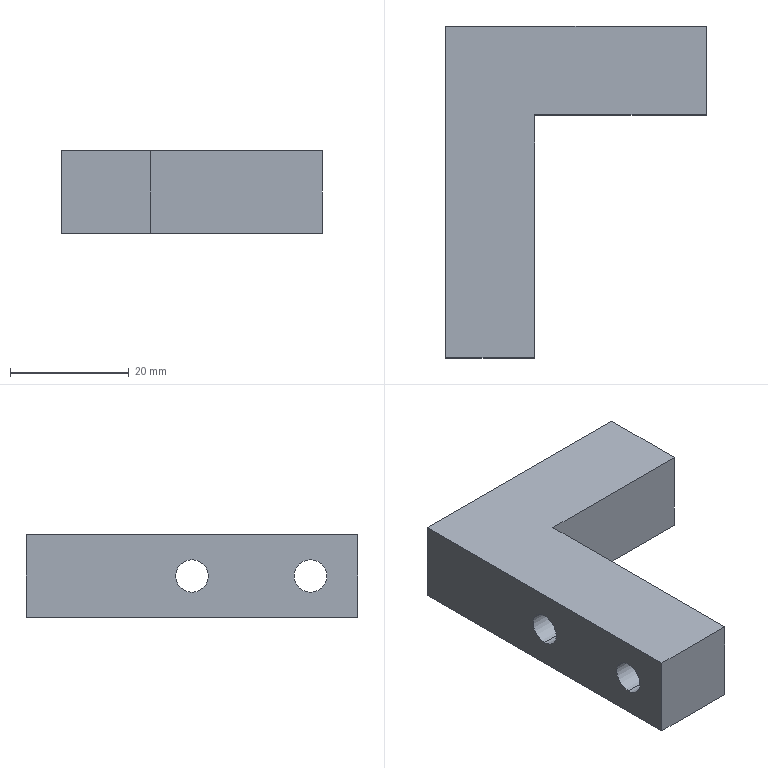Part | STEP file | PN_0017 fixing block | 1 solid | 20 faces | box 44 x 56 x 14 mm | volume 16926 mm3 | cylinder 8 | plane 8 | cone 4 | commonest cylinder face diameters 3.3 x4 5.5 x4
STEP:
#1=CARTESIAN_POINT('',(0.,0.,0.));
#2=DIRECTION('',(0.,0.,1.));
#3=DIRECTION('',(1.,0.,0.));
#4=AXIS2_PLACEMENT_3D('',#1,#2,#3);
#5=CARTESIAN_POINT('',(9.,44.,1.65));
#6=VERTEX_POINT('',#5);
#7=CARTESIAN_POINT('',(9.,56.,1.65));
#8=VERTEX_POINT('',#7);
#9=CARTESIAN_POINT('',(9.,56.,1.65));
#10=DIRECTION('',(0.,1.,0.));
#11=VECTOR('',#10,1.);
#12=LINE('',#9,#11);
#13=CARTESIAN_POINT('',(9.,56.,0.));
#14=DIRECTION('',(0.,1.,0.));
#15=DIRECTION('',(0.,0.,1.));
#16=AXIS2_PLACEMENT_3D('',#13,#14,#15);
#17=CYLINDRICAL_SURFACE('',#16,1.65);
#18=CARTESIAN_POINT('',(6.283,0.));
#19=DIRECTION('',(0.,1.));
#20=VECTOR('',#19,1.);
#21=LINE('',#18,#20);
#22=(GEOMETRIC_REPRESENTATION_CONTEXT(2)PARAMETRIC_REPRESENTATION_CONTEXT()REPRESENTATION_CONTEXT('',''));
#23=DEFINITIONAL_REPRESENTATION('',(#21),#22);
#24=PCURVE('',#17,#23);
#25=CARTESIAN_POINT('',(9.,56.,0.));
#26=DIRECTION('',(0.,1.,0.));
#27=DIRECTION('',(0.,0.,1.));
#28=AXIS2_PLACEMENT_3D('',#25,#26,#27);
#29=CYLINDRICAL_SURFACE('',#28,1.65);
#30=CARTESIAN_POINT('',(0.,0.));
#31=DIRECTION('',(0.,1.));
#32=VECTOR('',#31,1.);
#33=LINE('',#30,#32);
#34=(GEOMETRIC_REPRESENTATION_CONTEXT(2)PARAMETRIC_REPRESENTATION_CONTEXT()REPRESENTATION_CONTEXT('',''));
#35=DEFINITIONAL_REPRESENTATION('',(#33),#34);
#36=PCURVE('',#29,#35);
#37=SURFACE_CURVE('',#12,(#24,#36),.PCURVE_S1.);
#38=EDGE_CURVE('',#6,#8,#37,.T.);
#39=ORIENTED_EDGE('',*,*,#38,.T.);
#40=CARTESIAN_POINT('',(9.,56.,-1.65));
#41=VERTEX_POINT('',#40);
#42=CARTESIAN_POINT('',(9.,56.,0.));
#43=DIRECTION('',(0.,1.,0.));
#44=DIRECTION('',(0.,0.,1.));
#45=AXIS2_PLACEMENT_3D('',#42,#43,#44);
#46=CIRCLE('',#45,1.65);
#47=CARTESIAN_POINT('',(0.,0.));
#48=DIRECTION('',(1.,0.));
#49=VECTOR('',#48,1.);
#50=LINE('',#47,#49);
#51=(GEOMETRIC_REPRESENTATION_CONTEXT(2)PARAMETRIC_REPRESENTATION_CONTEXT()REPRESENTATION_CONTEXT('',''));
#52=DEFINITIONAL_REPRESENTATION('',(#50),#51);
#53=PCURVE('',#17,#52);
#54=CARTESIAN_POINT('',(0.,56.,7.));
#55=DIRECTION('',(0.,-1.,0.));
#56=DIRECTION('',(0.,0.,-1.));
#57=AXIS2_PLACEMENT_3D('',#54,#55,#56);
#58=PLANE('',#57);
#59=CARTESIAN_POINT('',(5.35,9.));
#60=CARTESIAN_POINT('',(5.35,11.858));
#61=CARTESIAN_POINT('',(7.825,10.429));
#62=CARTESIAN_POINT('',(10.3,9.));
#63=CARTESIAN_POINT('',(7.825,7.571));
#64=CARTESIAN_POINT('',(5.35,6.142));
#65=CARTESIAN_POINT('',(5.35,9.));
#66=(BOUNDED_CURVE()B_SPLINE_CURVE(2,(#59,#60,#61,#62,#63,#64,#65),.UNSPECIFIED.,.T.,.F.)B_SPLINE_CURVE_WITH_KNOTS((1,2,2,2,2,1),(-2.094,0.,2.094,4.189,6.283,8.378),.UNSPECIFIED.)CURVE()GEOMETRIC_REPRESENTATION_ITEM()RATIONAL_B_SPLINE_CURVE((1.,0.5,1.,0.5,1.,0.5,1.))REPRESENTATION_ITEM(''));
#67=(GEOMETRIC_REPRESENTATION_CONTEXT(2)PARAMETRIC_REPRESENTATION_CONTEXT()REPRESENTATION_CONTEXT('',''));
#68=DEFINITIONAL_REPRESENTATION('',(#66),#67);
#69=PCURVE('',#58,#68);
#70=SURFACE_CURVE('',#46,(#53,#69),.PCURVE_S1.);
#71=EDGE_CURVE('',#41,#8,#70,.T.);
#72=ORIENTED_EDGE('',*,*,#71,.F.);
#73=CARTESIAN_POINT('',(9.,44.,-1.65));
#74=VERTEX_POINT('',#73);
#75=CARTESIAN_POINT('',(9.,56.,-1.65));
#76=DIRECTION('',(0.,1.,0.));
#77=VECTOR('',#76,1.);
#78=LINE('',#75,#77);
#79=CARTESIAN_POINT('',(3.142,0.));
#80=DIRECTION('',(0.,1.));
#81=VECTOR('',#80,1.);
#82=LINE('',#79,#81);
#83=(GEOMETRIC_REPRESENTATION_CONTEXT(2)PARAMETRIC_REPRESENTATION_CONTEXT()REPRESENTATION_CONTEXT('',''));
#84=DEFINITIONAL_REPRESENTATION('',(#82),#83);
#85=PCURVE('',#17,#84);
#86=CARTESIAN_POINT('',(3.142,0.));
#87=DIRECTION('',(0.,1.));
#88=VECTOR('',#87,1.);
#89=LINE('',#86,#88);
#90=(GEOMETRIC_REPRESENTATION_CONTEXT(2)PARAMETRIC_REPRESENTATION_CONTEXT()REPRESENTATION_CONTEXT('',''));
#91=DEFINITIONAL_REPRESENTATION('',(#89),#90);
#92=PCURVE('',#29,#91);
#93=SURFACE_CURVE('',#78,(#85,#92),.PCURVE_S1.);
#94=EDGE_CURVE('',#74,#41,#93,.T.);
#95=ORIENTED_EDGE('',*,*,#94,.F.);
#96=CARTESIAN_POINT('',(9.,44.,0.));
#97=DIRECTION('',(0.,1.,0.));
#98=DIRECTION('',(0.,0.,1.));
#99=AXIS2_PLACEMENT_3D('',#96,#97,#98);
#100=CIRCLE('',#99,1.65);
#101=CARTESIAN_POINT('',(0.,-12.));
#102=DIRECTION('',(1.,0.));
#103=VECTOR('',#102,1.);
#104=LINE('',#101,#103);
#105=(GEOMETRIC_REPRESENTATION_CONTEXT(2)PARAMETRIC_REPRESENTATION_CONTEXT()REPRESENTATION_CONTEXT('',''));
#106=DEFINITIONAL_REPRESENTATION('',(#104),#105);
#107=PCURVE('',#17,#106);
#108=CARTESIAN_POINT('',(9.,44.,0.));
#109=DIRECTION('',(0.,1.,0.));
#110=DIRECTION('',(0.,0.,1.));
#111=AXIS2_PLACEMENT_3D('',#108,#109,#110);
#112=CONICAL_SURFACE('',#111,1.65,1.03);
#113=CARTESIAN_POINT('',(0.,0.));
#114=DIRECTION('',(1.,0.));
#115=VECTOR('',#114,1.);
#116=LINE('',#113,#115);
#117=(GEOMETRIC_REPRESENTATION_CONTEXT(2)PARAMETRIC_REPRESENTATION_CONTEXT()REPRESENTATION_CONTEXT('',''));
#118=DEFINITIONAL_REPRESENTATION('',(#116),#117);
#119=PCURVE('',#112,#118);
#120=SURFACE_CURVE('',#100,(#107,#119),.PCURVE_S1.);
#121=EDGE_CURVE('',#74,#6,#120,.T.);
#122=ORIENTED_EDGE('',*,*,#121,.T.);
#123=EDGE_LOOP('',(#39,#72,#95,#122));
#124=FACE_BOUND('',#123,.F.);
#125=ADVANCED_FACE('',(#124),#17,.F.);
#126=ORIENTED_EDGE('',*,*,#121,.F.);
#127=CARTESIAN_POINT('',(9.,43.009,0.));
#128=VERTEX_POINT('',#127);
#129=CARTESIAN_POINT('',(9.,44.,-1.65));
#130=DIRECTION('',(0.,0.515,-0.8572));
#131=VECTOR('',#130,1.);
#132=LINE('',#129,#131);
#133=CARTESIAN_POINT('',(3.142,0.));
#134=DIRECTION('',(0.,1.));
#135=VECTOR('',#134,1.);
#136=LINE('',#133,#135);
#137=(GEOMETRIC_REPRESENTATION_CONTEXT(2)PARAMETRIC_REPRESENTATION_CONTEXT()REPRESENTATION_CONTEXT('',''));
#138=DEFINITIONAL_REPRESENTATION('',(#136),#137);
#139=PCURVE('',#112,#138);
#140=CARTESIAN_POINT('',(9.,44.,0.));
#141=DIRECTION('',(0.,1.,0.));
#142=DIRECTION('',(0.,0.,1.));
#143=AXIS2_PLACEMENT_3D('',#140,#141,#142);
#144=CONICAL_SURFACE('',#143,1.65,1.03);
#145=CARTESIAN_POINT('',(3.142,0.));
#146=DIRECTION('',(0.,1.));
#147=VECTOR('',#146,1.);
#148=LINE('',#145,#147);
#149=(GEOMETRIC_REPRESENTATION_CONTEXT(2)PARAMETRIC_REPRESENTATION_CONTEXT()REPRESENTATION_CONTEXT('',''));
#150=DEFINITIONAL_REPRESENTATION('',(#148),#149);
#151=PCURVE('',#144,#150);
#152=SURFACE_CURVE('',#132,(#139,#151),.PCURVE_S1.);
#153=EDGE_CURVE('',#128,#74,#152,.T.);
#154=ORIENTED_EDGE('',*,*,#153,.F.);
#155=CARTESIAN_POINT('',(9.,44.,1.65));
#156=DIRECTION('',(0.,0.515,0.8572));
#157=VECTOR('',#156,1.);
#158=LINE('',#155,#157);
#159=CARTESIAN_POINT('',(6.283,0.));
#160=DIRECTION('',(0.,1.));
#161=VECTOR('',#160,1.);
#162=LINE('',#159,#161);
#163=(GEOMETRIC_REPRESENTATION_CONTEXT(2)PARAMETRIC_REPRESENTATION_CONTEXT()REPRESENTATION_CONTEXT('',''));
#164=DEFINITIONAL_REPRESENTATION('',(#162),#163);
#165=PCURVE('',#112,#164);
#166=CARTESIAN_POINT('',(0.,0.));
#167=DIRECTION('',(0.,1.));
#168=VECTOR('',#167,1.);
#169=LINE('',#166,#168);
#170=(GEOMETRIC_REPRESENTATION_CONTEXT(2)PARAMETRIC_REPRESENTATION_CONTEXT()REPRESENTATION_CONTEXT('',''));
#171=DEFINITIONAL_REPRESENTATION('',(#169),#170);
#172=PCURVE('',#144,#171);
#173=SURFACE_CURVE('',#158,(#165,#172),.PCURVE_S1.);
#174=EDGE_CURVE('',#128,#6,#173,.T.);
#175=ORIENTED_EDGE('',*,*,#174,.T.);
#176=EDGE_LOOP('',(#126,#154,#175));
#177=FACE_BOUND('',#176,.F.);
#178=ADVANCED_FACE('',(#177),#112,.F.);
#179=CARTESIAN_POINT('',(29.,44.,1.65));
#180=VERTEX_POINT('',#179);
#181=CARTESIAN_POINT('',(29.,56.,1.65));
#182=VERTEX_POINT('',#181);
#183=CARTESIAN_POINT('',(29.,56.,1.65));
#184=DIRECTION('',(0.,1.,0.));
#185=VECTOR('',#184,1.);
#186=LINE('',#183,#185);
#187=CARTESIAN_POINT('',(29.,56.,0.));
#188=DIRECTION('',(0.,1.,0.));
#189=DIRECTION('',(0.,0.,1.));
#190=AXIS2_PLACEMENT_3D('',#187,#188,#189);
#191=CYLINDRICAL_SURFACE('',#190,1.65);
#192=CARTESIAN_POINT('',(6.283,0.));
#193=DIRECTION('',(0.,1.));
#194=VECTOR('',#193,1.);
#195=LINE('',#192,#194);
#196=(GEOMETRIC_REPRESENTATION_CONTEXT(2)PARAMETRIC_REPRESENTATION_CONTEXT()REPRESENTATION_CONTEXT('',''));
#197=DEFINITIONAL_REPRESENTATION('',(#195),#196);
#198=PCURVE('',#191,#197);
#199=CARTESIAN_POINT('',(29.,56.,0.));
#200=DIRECTION('',(0.,1.,0.));
#201=DIRECTION('',(0.,0.,1.));
#202=AXIS2_PLACEMENT_3D('',#199,#200,#201);
#203=CYLINDRICAL_SURFACE('',#202,1.65);
#204=CARTESIAN_POINT('',(0.,0.));
#205=DIRECTION('',(0.,1.));
#206=VECTOR('',#205,1.);
#207=LINE('',#204,#206);
#208=(GEOMETRIC_REPRESENTATION_CONTEXT(2)PARAMETRIC_REPRESENTATION_CONTEXT()REPRESENTATION_CONTEXT('',''));
#209=DEFINITIONAL_REPRESENTATION('',(#207),#208);
#210=PCURVE('',#203,#209);
#211=SURFACE_CURVE('',#186,(#198,#210),.PCURVE_S1.);
#212=EDGE_CURVE('',#180,#182,#211,.T.);
#213=ORIENTED_EDGE('',*,*,#212,.T.);
#214=CARTESIAN_POINT('',(29.,56.,-1.65));
#215=VERTEX_POINT('',#214);
#216=CARTESIAN_POINT('',(29.,56.,0.));
#217=DIRECTION('',(0.,1.,0.));
#218=DIRECTION('',(0.,0.,1.));
#219=AXIS2_PLACEMENT_3D('',#216,#217,#218);
#220=CIRCLE('',#219,1.65);
#221=CARTESIAN_POINT('',(0.,0.));
#222=DIRECTION('',(1.,0.));
#223=VECTOR('',#222,1.);
#224=LINE('',#221,#223);
#225=(GEOMETRIC_REPRESENTATION_CONTEXT(2)PARAMETRIC_REPRESENTATION_CONTEXT()REPRESENTATION_CONTEXT('',''));
#226=DEFINITIONAL_REPRESENTATION('',(#224),#225);
#227=PCURVE('',#191,#226);
#228=CARTESIAN_POINT('',(5.35,29.));
#229=CARTESIAN_POINT('',(5.35,31.858));
#230=CARTESIAN_POINT('',(7.825,30.429));
#231=CARTESIAN_POINT('',(10.3,29.));
#232=CARTESIAN_POINT('',(7.825,27.571));
#233=CARTESIAN_POINT('',(5.35,26.142));
#234=CARTESIAN_POINT('',(5.35,29.));
#235=(BOUNDED_CURVE()B_SPLINE_CURVE(2,(#228,#229,#230,#231,#232,#233,#234),.UNSPECIFIED.,.T.,.F.)B_SPLINE_CURVE_WITH_KNOTS((1,2,2,2,2,1),(-2.094,0.,2.094,4.189,6.283,8.378),.UNSPECIFIED.)CURVE()GEOMETRIC_REPRESENTATION_ITEM()RATIONAL_B_SPLINE_CURVE((1.,0.5,1.,0.5,1.,0.5,1.))REPRESENTATION_ITEM(''));
#236=(GEOMETRIC_REPRESENTATION_CONTEXT(2)PARAMETRIC_REPRESENTATION_CONTEXT()REPRESENTATION_CONTEXT('',''));
#237=DEFINITIONAL_REPRESENTATION('',(#235),#236);
#238=PCURVE('',#58,#237);
#239=SURFACE_CURVE('',#220,(#227,#238),.PCURVE_S1.);
#240=EDGE_CURVE('',#215,#182,#239,.T.);
#241=ORIENTED_EDGE('',*,*,#240,.F.);
#242=CARTESIAN_POINT('',(29.,44.,-1.65));
#243=VERTEX_POINT('',#242);
#244=CARTESIAN_POINT('',(29.,56.,-1.65));
#245=DIRECTION('',(0.,1.,0.));
#246=VECTOR('',#245,1.);
#247=LINE('',#244,#246);
#248=CARTESIAN_POINT('',(3.142,0.));
#249=DIRECTION('',(0.,1.));
#250=VECTOR('',#249,1.);
#251=LINE('',#248,#250);
#252=(GEOMETRIC_REPRESENTATION_CONTEXT(2)PARAMETRIC_REPRESENTATION_CONTEXT()REPRESENTATION_CONTEXT('',''));
#253=DEFINITIONAL_REPRESENTATION('',(#251),#252);
#254=PCURVE('',#191,#253);
#255=CARTESIAN_POINT('',(3.142,0.));
#256=DIRECTION('',(0.,1.));
#257=VECTOR('',#256,1.);
#258=LINE('',#255,#257);
#259=(GEOMETRIC_REPRESENTATION_CONTEXT(2)PARAMETRIC_REPRESENTATION_CONTEXT()REPRESENTATION_CONTEXT('',''));
#260=DEFINITIONAL_REPRESENTATION('',(#258),#259);
#261=PCURVE('',#203,#260);
#262=SURFACE_CURVE('',#247,(#254,#261),.PCURVE_S1.);
#263=EDGE_CURVE('',#243,#215,#262,.T.);
#264=ORIENTED_EDGE('',*,*,#263,.F.);
#265=CARTESIAN_POINT('',(29.,44.,0.));
#266=DIRECTION('',(0.,1.,0.));
#267=DIRECTION('',(0.,0.,1.));
#268=AXIS2_PLACEMENT_3D('',#265,#266,#267);
#269=CIRCLE('',#268,1.65);
#270=CARTESIAN_POINT('',(0.,-12.));
#271=DIRECTION('',(1.,0.));
#272=VECTOR('',#271,1.);
#273=LINE('',#270,#272);
#274=(GEOMETRIC_REPRESENTATION_CONTEXT(2)PARAMETRIC_REPRESENTATION_CONTEXT()REPRESENTATION_CONTEXT('',''));
#275=DEFINITIONAL_REPRESENTATION('',(#273),#274);
#276=PCURVE('',#191,#275);
#277=CARTESIAN_POINT('',(29.,44.,0.));
#278=DIRECTION('',(0.,1.,0.));
#279=DIRECTION('',(0.,0.,1.));
#280=AXIS2_PLACEMENT_3D('',#277,#278,#279);
#281=CONICAL_SURFACE('',#280,1.65,1.03);
#282=CARTESIAN_POINT('',(0.,0.));
#283=DIRECTION('',(1.,0.));
#284=VECTOR('',#283,1.);
#285=LINE('',#282,#284);
#286=(GEOMETRIC_REPRESENTATION_CONTEXT(2)PARAMETRIC_REPRESENTATION_CONTEXT()REPRESENTATION_CONTEXT('',''));
#287=DEFINITIONAL_REPRESENTATION('',(#285),#286);
#288=PCURVE('',#281,#287);
#289=SURFACE_CURVE('',#269,(#276,#288),.PCURVE_S1.);
#290=EDGE_CURVE('',#243,#180,#289,.T.);
#291=ORIENTED_EDGE('',*,*,#290,.T.);
#292=EDGE_LOOP('',(#213,#241,#264,#291));
#293=FACE_BOUND('',#292,.F.);
#294=ADVANCED_FACE('',(#293),#191,.F.);
#295=ORIENTED_EDGE('',*,*,#290,.F.);
#296=CARTESIAN_POINT('',(29.,43.009,0.));
#297=VERTEX_POINT('',#296);
#298=CARTESIAN_POINT('',(29.,44.,-1.65));
#299=DIRECTION('',(0.,0.515,-0.8572));
#300=VECTOR('',#299,1.);
#301=LINE('',#298,#300);
#302=CARTESIAN_POINT('',(3.142,0.));
#303=DIRECTION('',(0.,1.));
#304=VECTOR('',#303,1.);
#305=LINE('',#302,#304);
#306=(GEOMETRIC_REPRESENTATION_CONTEXT(2)PARAMETRIC_REPRESENTATION_CONTEXT()REPRESENTATION_CONTEXT('',''));
#307=DEFINITIONAL_REPRESENTATION('',(#305),#306);
#308=PCURVE('',#281,#307);
#309=CARTESIAN_POINT('',(29.,44.,0.));
#310=DIRECTION('',(0.,1.,0.));
#311=DIRECTION('',(0.,0.,1.));
#312=AXIS2_PLACEMENT_3D('',#309,#310,#311);
#313=CONICAL_SURFACE('',#312,1.65,1.03);
#314=CARTESIAN_POINT('',(3.142,0.));
#315=DIRECTION('',(0.,1.));
#316=VECTOR('',#315,1.);
#317=LINE('',#314,#316);
#318=(GEOMETRIC_REPRESENTATION_CONTEXT(2)PARAMETRIC_REPRESENTATION_CONTEXT()REPRESENTATION_CONTEXT('',''));
#319=DEFINITIONAL_REPRESENTATION('',(#317),#318);
#320=PCURVE('',#313,#319);
#321=SURFACE_CURVE('',#301,(#308,#320),.PCURVE_S1.);
#322=EDGE_CURVE('',#297,#243,#321,.T.);
#323=ORIENTED_EDGE('',*,*,#322,.F.);
#324=CARTESIAN_POINT('',(29.,44.,1.65));
#325=DIRECTION('',(0.,0.515,0.8572));
#326=VECTOR('',#325,1.);
#327=LINE('',#324,#326);
#328=CARTESIAN_POINT('',(6.283,0.));
#329=DIRECTION('',(0.,1.));
#330=VECTOR('',#329,1.);
#331=LINE('',#328,#330);
#332=(GEOMETRIC_REPRESENTATION_CONTEXT(2)PARAMETRIC_REPRESENTATION_CONTEXT()REPRESENTATION_CONTEXT('',''));
#333=DEFINITIONAL_REPRESENTATION('',(#331),#332);
#334=PCURVE('',#281,#333);
#335=CARTESIAN_POINT('',(0.,0.));
#336=DIRECTION('',(0.,1.));
#337=VECTOR('',#336,1.);
#338=LINE('',#335,#337);
#339=(GEOMETRIC_REPRESENTATION_CONTEXT(2)PARAMETRIC_REPRESENTATION_CONTEXT()REPRESENTATION_CONTEXT('',''));
#340=DEFINITIONAL_REPRESENTATION('',(#338),#339);
#341=PCURVE('',#313,#340);
#342=SURFACE_CURVE('',#327,(#334,#341),.PCURVE_S1.);
#343=EDGE_CURVE('',#297,#180,#342,.T.);
#344=ORIENTED_EDGE('',*,*,#343,.T.);
#345=EDGE_LOOP('',(#295,#323,#344));
#346=FACE_BOUND('',#345,.F.);
#347=ADVANCED_FACE('',(#346),#281,.F.);
#348=CARTESIAN_POINT('',(0.,8.,-2.75));
#349=VERTEX_POINT('',#348);
#350=CARTESIAN_POINT('',(15.,8.,-2.75));
#351=VERTEX_POINT('',#350);
#352=CARTESIAN_POINT('',(15.,8.,-2.75));
#353=DIRECTION('',(1.,0.,0.));
#354=VECTOR('',#353,1.);
#355=LINE('',#352,#354);
#356=CARTESIAN_POINT('',(15.,8.,0.));
#357=DIRECTION('',(1.,0.,0.));
#358=DIRECTION('',(0.,0.,-1.));
#359=AXIS2_PLACEMENT_3D('',#356,#357,#358);
#360=CYLINDRICAL_SURFACE('',#359,2.75);
#361=CARTESIAN_POINT('',(6.283,0.));
#362=DIRECTION('',(0.,1.));
#363=VECTOR('',#362,1.);
#364=LINE('',#361,#363);
#365=(GEOMETRIC_REPRESENTATION_CONTEXT(2)PARAMETRIC_REPRESENTATION_CONTEXT()REPRESENTATION_CONTEXT('',''));
#366=DEFINITIONAL_REPRESENTATION('',(#364),#365);
#367=PCURVE('',#360,#366);
#368=CARTESIAN_POINT('',(15.,8.,0.));
#369=DIRECTION('',(1.,0.,0.));
#370=DIRECTION('',(0.,0.,-1.));
#371=AXIS2_PLACEMENT_3D('',#368,#369,#370);
#372=CYLINDRICAL_SURFACE('',#371,2.75);
#373=CARTESIAN_POINT('',(0.,0.));
#374=DIRECTION('',(0.,1.));
#375=VECTOR('',#374,1.);
#376=LINE('',#373,#375);
#377=(GEOMETRIC_REPRESENTATION_CONTEXT(2)PARAMETRIC_REPRESENTATION_CONTEXT()REPRESENTATION_CONTEXT('',''));
#378=DEFINITIONAL_REPRESENTATION('',(#376),#377);
#379=PCURVE('',#372,#378);
#380=SURFACE_CURVE('',#355,(#367,#379),.PCURVE_S1.);
#381=EDGE_CURVE('',#349,#351,#380,.T.);
#382=ORIENTED_EDGE('',*,*,#381,.T.);
#383=CARTESIAN_POINT('',(15.,8.,2.75));
#384=VERTEX_POINT('',#383);
#385=CARTESIAN_POINT('',(15.,8.,0.));
#386=DIRECTION('',(1.,0.,0.));
#387=DIRECTION('',(0.,0.,-1.));
#388=AXIS2_PLACEMENT_3D('',#385,#386,#387);
#389=CIRCLE('',#388,2.75);
#390=CARTESIAN_POINT('',(0.,0.));
#391=DIRECTION('',(1.,0.));
#392=VECTOR('',#391,1.);
#393=LINE('',#390,#392);
#394=(GEOMETRIC_REPRESENTATION_CONTEXT(2)PARAMETRIC_REPRESENTATION_CONTEXT()REPRESENTATION_CONTEXT('',''));
#395=DEFINITIONAL_REPRESENTATION('',(#393),#394);
#396=PCURVE('',#360,#395);
#397=CARTESIAN_POINT('',(15.,41.,7.));
#398=DIRECTION('',(-1.,0.,0.));
#399=DIRECTION('',(0.,-1.,0.));
#400=AXIS2_PLACEMENT_3D('',#397,#398,#399);
#401=PLANE('',#400);
#402=CARTESIAN_POINT('',(33.,-9.75));
#403=CARTESIAN_POINT('',(28.237,-9.75));
#404=CARTESIAN_POINT('',(30.618,-5.625));
#405=CARTESIAN_POINT('',(33.,-1.5));
#406=CARTESIAN_POINT('',(35.382,-5.625));
#407=CARTESIAN_POINT('',(37.763,-9.75));
#408=CARTESIAN_POINT('',(33.,-9.75));
#409=(BOUNDED_CURVE()B_SPLINE_CURVE(2,(#402,#403,#404,#405,#406,#407,#408),.UNSPECIFIED.,.T.,.F.)B_SPLINE_CURVE_WITH_KNOTS((1,2,2,2,2,1),(-2.094,0.,2.094,4.189,6.283,8.378),.UNSPECIFIED.)CURVE()GEOMETRIC_REPRESENTATION_ITEM()RATIONAL_B_SPLINE_CURVE((1.,0.5,1.,0.5,1.,0.5,1.))REPRESENTATION_ITEM(''));
#410=(GEOMETRIC_REPRESENTATION_CONTEXT(2)PARAMETRIC_REPRESENTATION_CONTEXT()REPRESENTATION_CONTEXT('',''));
#411=DEFINITIONAL_REPRESENTATION('',(#409),#410);
#412=PCURVE('',#401,#411);
#413=SURFACE_CURVE('',#389,(#396,#412),.PCURVE_S1.);
#414=EDGE_CURVE('',#384,#351,#413,.T.);
#415=ORIENTED_EDGE('',*,*,#414,.F.);
#416=CARTESIAN_POINT('',(0.,8.,2.75));
#417=VERTEX_POINT('',#416);
#418=CARTESIAN_POINT('',(15.,8.,2.75));
#419=DIRECTION('',(1.,0.,0.));
#420=VECTOR('',#419,1.);
#421=LINE('',#418,#420);
#422=CARTESIAN_POINT('',(3.142,0.));
#423=DIRECTION('',(0.,1.));
#424=VECTOR('',#423,1.);
#425=LINE('',#422,#424);
#426=(GEOMETRIC_REPRESENTATION_CONTEXT(2)PARAMETRIC_REPRESENTATION_CONTEXT()REPRESENTATION_CONTEXT('',''));
#427=DEFINITIONAL_REPRESENTATION('',(#425),#426);
#428=PCURVE('',#360,#427);
#429=CARTESIAN_POINT('',(3.142,0.));
#430=DIRECTION('',(0.,1.));
#431=VECTOR('',#430,1.);
#432=LINE('',#429,#431);
#433=(GEOMETRIC_REPRESENTATION_CONTEXT(2)PARAMETRIC_REPRESENTATION_CONTEXT()REPRESENTATION_CONTEXT('',''));
#434=DEFINITIONAL_REPRESENTATION('',(#432),#433);
#435=PCURVE('',#372,#434);
#436=SURFACE_CURVE('',#421,(#428,#435),.PCURVE_S1.);
#437=EDGE_CURVE('',#417,#384,#436,.T.);
#438=ORIENTED_EDGE('',*,*,#437,.F.);
#439=CARTESIAN_POINT('',(0.,8.,0.));
#440=DIRECTION('',(1.,0.,0.));
#441=DIRECTION('',(0.,0.,-1.));
#442=AXIS2_PLACEMENT_3D('',#439,#440,#441);
#443=CIRCLE('',#442,2.75);
#444=CARTESIAN_POINT('',(0.,-15.));
#445=DIRECTION('',(1.,0.));
#446=VECTOR('',#445,1.);
#447=LINE('',#444,#446);
#448=(GEOMETRIC_REPRESENTATION_CONTEXT(2)PARAMETRIC_REPRESENTATION_CONTEXT()REPRESENTATION_CONTEXT('',''));
#449=DEFINITIONAL_REPRESENTATION('',(#447),#448);
#450=PCURVE('',#360,#449);
#451=CARTESIAN_POINT('',(0.,0.,7.));
#452=DIRECTION('',(1.,0.,0.));
#453=DIRECTION('',(0.,0.,-1.));
#454=AXIS2_PLACEMENT_3D('',#451,#452,#453);
#455=PLANE('',#454);
#456=CARTESIAN_POINT('',(7.,8.));
#457=DIRECTION('',(1.,0.));
#458=AXIS2_PLACEMENT_2D('',#456,#457);
#459=CIRCLE('',#458,2.75);
#460=(GEOMETRIC_REPRESENTATION_CONTEXT(2)PARAMETRIC_REPRESENTATION_CONTEXT()REPRESENTATION_CONTEXT('',''));
#461=DEFINITIONAL_REPRESENTATION('',(#459),#460);
#462=PCURVE('',#455,#461);
#463=SURFACE_CURVE('',#443,(#450,#462),.PCURVE_S1.);
#464=EDGE_CURVE('',#417,#349,#463,.T.);
#465=ORIENTED_EDGE('',*,*,#464,.T.);
#466=EDGE_LOOP('',(#382,#415,#438,#465));
#467=FACE_BOUND('',#466,.F.);
#468=ADVANCED_FACE('',(#467),#360,.F.);
#469=CARTESIAN_POINT('',(0.,28.,-2.75));
#470=VERTEX_POINT('',#469);
#471=CARTESIAN_POINT('',(15.,28.,-2.75));
#472=VERTEX_POINT('',#471);
#473=CARTESIAN_POINT('',(15.,28.,-2.75));
#474=DIRECTION('',(1.,0.,0.));
#475=VECTOR('',#474,1.);
#476=LINE('',#473,#475);
#477=CARTESIAN_POINT('',(15.,28.,0.));
#478=DIRECTION('',(1.,0.,0.));
#479=DIRECTION('',(0.,0.,-1.));
#480=AXIS2_PLACEMENT_3D('',#477,#478,#479);
#481=CYLINDRICAL_SURFACE('',#480,2.75);
#482=CARTESIAN_POINT('',(6.283,0.));
#483=DIRECTION('',(0.,1.));
#484=VECTOR('',#483,1.);
#485=LINE('',#482,#484);
#486=(GEOMETRIC_REPRESENTATION_CONTEXT(2)PARAMETRIC_REPRESENTATION_CONTEXT()REPRESENTATION_CONTEXT('',''));
#487=DEFINITIONAL_REPRESENTATION('',(#485),#486);
#488=PCURVE('',#481,#487);
#489=CARTESIAN_POINT('',(15.,28.,0.));
#490=DIRECTION('',(1.,0.,0.));
#491=DIRECTION('',(0.,0.,-1.));
#492=AXIS2_PLACEMENT_3D('',#489,#490,#491);
#493=CYLINDRICAL_SURFACE('',#492,2.75);
#494=CARTESIAN_POINT('',(0.,0.));
#495=DIRECTION('',(0.,1.));
#496=VECTOR('',#495,1.);
#497=LINE('',#494,#496);
#498=(GEOMETRIC_REPRESENTATION_CONTEXT(2)PARAMETRIC_REPRESENTATION_CONTEXT()REPRESENTATION_CONTEXT('',''));
#499=DEFINITIONAL_REPRESENTATION('',(#497),#498);
#500=PCURVE('',#493,#499);
#501=SURFACE_CURVE('',#476,(#488,#500),.PCURVE_S1.);
#502=EDGE_CURVE('',#470,#472,#501,.T.);
#503=ORIENTED_EDGE('',*,*,#502,.T.);
#504=CARTESIAN_POINT('',(15.,28.,2.75));
#505=VERTEX_POINT('',#504);
#506=CARTESIAN_POINT('',(15.,28.,0.));
#507=DIRECTION('',(1.,0.,0.));
#508=DIRECTION('',(0.,0.,-1.));
#509=AXIS2_PLACEMENT_3D('',#506,#507,#508);
#510=CIRCLE('',#509,2.75);
#511=CARTESIAN_POINT('',(0.,0.));
#512=DIRECTION('',(1.,0.));
#513=VECTOR('',#512,1.);
#514=LINE('',#511,#513);
#515=(GEOMETRIC_REPRESENTATION_CONTEXT(2)PARAMETRIC_REPRESENTATION_CONTEXT()REPRESENTATION_CONTEXT('',''));
#516=DEFINITIONAL_REPRESENTATION('',(#514),#515);
#517=PCURVE('',#481,#516);
#518=CARTESIAN_POINT('',(13.,-9.75));
#519=CARTESIAN_POINT('',(8.237,-9.75));
#520=CARTESIAN_POINT('',(10.618,-5.625));
#521=CARTESIAN_POINT('',(13.,-1.5));
#522=CARTESIAN_POINT('',(15.382,-5.625));
#523=CARTESIAN_POINT('',(17.763,-9.75));
#524=CARTESIAN_POINT('',(13.,-9.75));
#525=(BOUNDED_CURVE()B_SPLINE_CURVE(2,(#518,#519,#520,#521,#522,#523,#524),.UNSPECIFIED.,.T.,.F.)B_SPLINE_CURVE_WITH_KNOTS((1,2,2,2,2,1),(-2.094,0.,2.094,4.189,6.283,8.378),.UNSPECIFIED.)CURVE()GEOMETRIC_REPRESENTATION_ITEM()RATIONAL_B_SPLINE_CURVE((1.,0.5,1.,0.5,1.,0.5,1.))REPRESENTATION_ITEM(''));
#526=(GEOMETRIC_REPRESENTATION_CONTEXT(2)PARAMETRIC_REPRESENTATION_CONTEXT()REPRESENTATION_CONTEXT('',''));
#527=DEFINITIONAL_REPRESENTATION('',(#525),#526);
#528=PCURVE('',#401,#527);
#529=SURFACE_CURVE('',#510,(#517,#528),.PCURVE_S1.);
#530=EDGE_CURVE('',#505,#472,#529,.T.);
#531=ORIENTED_EDGE('',*,*,#530,.F.);
#532=CARTESIAN_POINT('',(0.,28.,2.75));
#533=VERTEX_POINT('',#532);
#534=CARTESIAN_POINT('',(15.,28.,2.75));
#535=DIRECTION('',(1.,0.,0.));
#536=VECTOR('',#535,1.);
#537=LINE('',#534,#536);
#538=CARTESIAN_POINT('',(3.142,0.));
#539=DIRECTION('',(0.,1.));
#540=VECTOR('',#539,1.);
#541=LINE('',#538,#540);
#542=(GEOMETRIC_REPRESENTATION_CONTEXT(2)PARAMETRIC_REPRESENTATION_CONTEXT()REPRESENTATION_CONTEXT('',''));
#543=DEFINITIONAL_REPRESENTATION('',(#541),#542);
#544=PCURVE('',#481,#543);
#545=CARTESIAN_POINT('',(3.142,0.));
#546=DIRECTION('',(0.,1.));
#547=VECTOR('',#546,1.);
#548=LINE('',#545,#547);
#549=(GEOMETRIC_REPRESENTATION_CONTEXT(2)PARAMETRIC_REPRESENTATION_CONTEXT()REPRESENTATION_CONTEXT('',''));
#550=DEFINITIONAL_REPRESENTATION('',(#548),#549);
#551=PCURVE('',#493,#550);
#552=SURFACE_CURVE('',#537,(#544,#551),.PCURVE_S1.);
#553=EDGE_CURVE('',#533,#505,#552,.T.);
#554=ORIENTED_EDGE('',*,*,#553,.F.);
#555=CARTESIAN_POINT('',(0.,28.,0.));
#556=DIRECTION('',(1.,0.,0.));
#557=DIRECTION('',(0.,0.,-1.));
#558=AXIS2_PLACEMENT_3D('',#555,#556,#557);
#559=CIRCLE('',#558,2.75);
#560=CARTESIAN_POINT('',(0.,-15.));
#561=DIRECTION('',(1.,0.));
#562=VECTOR('',#561,1.);
#563=LINE('',#560,#562);
#564=(GEOMETRIC_REPRESENTATION_CONTEXT(2)PARAMETRIC_REPRESENTATION_CONTEXT()REPRESENTATION_CONTEXT('',''));
#565=DEFINITIONAL_REPRESENTATION('',(#563),#564);
#566=PCURVE('',#481,#565);
#567=CARTESIAN_POINT('',(7.,28.));
#568=DIRECTION('',(1.,0.));
#569=AXIS2_PLACEMENT_2D('',#567,#568);
#570=CIRCLE('',#569,2.75);
#571=(GEOMETRIC_REPRESENTATION_CONTEXT(2)PARAMETRIC_REPRESENTATION_CONTEXT()REPRESENTATION_CONTEXT('',''));
#572=DEFINITIONAL_REPRESENTATION('',(#570),#571);
#573=PCURVE('',#455,#572);
#574=SURFACE_CURVE('',#559,(#566,#573),.PCURVE_S1.);
#575=EDGE_CURVE('',#533,#470,#574,.T.);
#576=ORIENTED_EDGE('',*,*,#575,.T.);
#577=EDGE_LOOP('',(#503,#531,#554,#576));
#578=FACE_BOUND('',#577,.F.);
#579=ADVANCED_FACE('',(#578),#481,.F.);
#580=CARTESIAN_POINT('',(0.,0.,-7.));
#581=VERTEX_POINT('',#580);
#582=CARTESIAN_POINT('',(15.,0.,-7.));
#583=VERTEX_POINT('',#582);
#584=CARTESIAN_POINT('',(15.,0.,-7.));
#585=DIRECTION('',(1.,0.,0.));
#586=VECTOR('',#585,1.);
#587=LINE('',#584,#586);
#588=CARTESIAN_POINT('',(15.,0.,7.));
#589=DIRECTION('',(0.,1.,0.));
#590=DIRECTION('',(-1.,0.,0.));
#591=AXIS2_PLACEMENT_3D('',#588,#589,#590);
#592=PLANE('',#591);
#593=CARTESIAN_POINT('',(0.,-14.));
#594=DIRECTION('',(-1.,0.));
#595=VECTOR('',#594,1.);
#596=LINE('',#593,#595);
#597=(GEOMETRIC_REPRESENTATION_CONTEXT(2)PARAMETRIC_REPRESENTATION_CONTEXT()REPRESENTATION_CONTEXT('',''));
#598=DEFINITIONAL_REPRESENTATION('',(#596),#597);
#599=PCURVE('',#592,#598);
#600=CARTESIAN_POINT('',(0.,0.,-7.));
#601=DIRECTION('',(0.,0.,-1.));
#602=DIRECTION('',(-1.,0.,0.));
#603=AXIS2_PLACEMENT_3D('',#600,#601,#602);
#604=PLANE('',#603);
#605=CARTESIAN_POINT('',(-15.,0.));
#606=DIRECTION('',(-1.,0.));
#607=VECTOR('',#606,1.);
#608=LINE('',#605,#607);
#609=(GEOMETRIC_REPRESENTATION_CONTEXT(2)PARAMETRIC_REPRESENTATION_CONTEXT()REPRESENTATION_CONTEXT('',''));
#610=DEFINITIONAL_REPRESENTATION('',(#608),#609);
#611=PCURVE('',#604,#610);
#612=SURFACE_CURVE('',#587,(#599,#611),.PCURVE_S1.);
#613=EDGE_CURVE('',#581,#583,#612,.T.);
#614=ORIENTED_EDGE('',*,*,#613,.T.);
#615=CARTESIAN_POINT('',(15.,0.,7.));
#616=VERTEX_POINT('',#615);
#617=CARTESIAN_POINT('',(15.,0.,7.));
#618=DIRECTION('',(0.,0.,-1.));
#619=VECTOR('',#618,1.);
#620=LINE('',#617,#619);
#621=CARTESIAN_POINT('',(0.,0.));
#622=DIRECTION('',(0.,-1.));
#623=VECTOR('',#622,1.);
#624=LINE('',#621,#623);
#625=(GEOMETRIC_REPRESENTATION_CONTEXT(2)PARAMETRIC_REPRESENTATION_CONTEXT()REPRESENTATION_CONTEXT('',''));
#626=DEFINITIONAL_REPRESENTATION('',(#624),#625);
#627=PCURVE('',#592,#626);
#628=CARTESIAN_POINT('',(41.,0.));
#629=DIRECTION('',(0.,-1.));
#630=VECTOR('',#629,1.);
#631=LINE('',#628,#630);
#632=(GEOMETRIC_REPRESENTATION_CONTEXT(2)PARAMETRIC_REPRESENTATION_CONTEXT()REPRESENTATION_CONTEXT('',''));
#633=DEFINITIONAL_REPRESENTATION('',(#631),#632);
#634=PCURVE('',#401,#633);
#635=SURFACE_CURVE('',#620,(#627,#634),.PCURVE_S1.);
#636=EDGE_CURVE('',#616,#583,#635,.T.);
#637=ORIENTED_EDGE('',*,*,#636,.F.);
#638=CARTESIAN_POINT('',(0.,0.,7.));
#639=VERTEX_POINT('',#638);
#640=CARTESIAN_POINT('',(15.,0.,7.));
#641=DIRECTION('',(1.,0.,0.));
#642=VECTOR('',#641,1.);
#643=LINE('',#640,#642);
#644=CARTESIAN_POINT('',(0.,0.));
#645=DIRECTION('',(-1.,0.));
#646=VECTOR('',#645,1.);
#647=LINE('',#644,#646);
#648=(GEOMETRIC_REPRESENTATION_CONTEXT(2)PARAMETRIC_REPRESENTATION_CONTEXT()REPRESENTATION_CONTEXT('',''));
#649=DEFINITIONAL_REPRESENTATION('',(#647),#648);
#650=PCURVE('',#592,#649);
#651=CARTESIAN_POINT('',(0.,0.,7.));
#652=DIRECTION('',(0.,0.,-1.));
#653=DIRECTION('',(-1.,0.,0.));
#654=AXIS2_PLACEMENT_3D('',#651,#652,#653);
#655=PLANE('',#654);
#656=CARTESIAN_POINT('',(-15.,0.));
#657=DIRECTION('',(-1.,0.));
#658=VECTOR('',#657,1.);
#659=LINE('',#656,#658);
#660=(GEOMETRIC_REPRESENTATION_CONTEXT(2)PARAMETRIC_REPRESENTATION_CONTEXT()REPRESENTATION_CONTEXT('',''));
#661=DEFINITIONAL_REPRESENTATION('',(#659),#660);
#662=PCURVE('',#655,#661);
#663=SURFACE_CURVE('',#643,(#650,#662),.PCURVE_S1.);
#664=EDGE_CURVE('',#639,#616,#663,.T.);
#665=ORIENTED_EDGE('',*,*,#664,.F.);
#666=CARTESIAN_POINT('',(0.,0.,7.));
#667=DIRECTION('',(0.,0.,-1.));
#668=VECTOR('',#667,1.);
#669=LINE('',#666,#668);
#670=CARTESIAN_POINT('',(15.,0.));
#671=DIRECTION('',(0.,-1.));
#672=VECTOR('',#671,1.);
#673=LINE('',#670,#672);
#674=(GEOMETRIC_REPRESENTATION_CONTEXT(2)PARAMETRIC_REPRESENTATION_CONTEXT()REPRESENTATION_CONTEXT('',''));
#675=DEFINITIONAL_REPRESENTATION('',(#673),#674);
#676=PCURVE('',#592,#675);
#677=CARTESIAN_POINT('',(0.,0.));
#678=DIRECTION('',(1.,0.));
#679=VECTOR('',#678,1.);
#680=LINE('',#677,#679);
#681=(GEOMETRIC_REPRESENTATION_CONTEXT(2)PARAMETRIC_REPRESENTATION_CONTEXT()REPRESENTATION_CONTEXT('',''));
#682=DEFINITIONAL_REPRESENTATION('',(#680),#681);
#683=PCURVE('',#455,#682);
#684=SURFACE_CURVE('',#669,(#676,#683),.PCURVE_S1.);
#685=EDGE_CURVE('',#639,#581,#684,.T.);
#686=ORIENTED_EDGE('',*,*,#685,.T.);
#687=EDGE_LOOP('',(#614,#637,#665,#686));
#688=FACE_BOUND('',#687,.T.);
#689=ADVANCED_FACE('',(#688),#592,.F.);
#690=CARTESIAN_POINT('',(15.,8.,0.));
#691=DIRECTION('',(1.,0.,0.));
#692=DIRECTION('',(0.,0.,-1.));
#693=AXIS2_PLACEMENT_3D('',#690,#691,#692);
#694=CIRCLE('',#693,2.75);
#695=CARTESIAN_POINT('',(33.,-9.75));
#696=CARTESIAN_POINT('',(28.237,-9.75));
#697=CARTESIAN_POINT('',(30.618,-5.625));
#698=CARTESIAN_POINT('',(33.,-1.5));
#699=CARTESIAN_POINT('',(35.382,-5.625));
#700=CARTESIAN_POINT('',(37.763,-9.75));
#701=CARTESIAN_POINT('',(33.,-9.75));
#702=(BOUNDED_CURVE()B_SPLINE_CURVE(2,(#695,#696,#697,#698,#699,#700,#701),.UNSPECIFIED.,.T.,.F.)B_SPLINE_CURVE_WITH_KNOTS((1,2,2,2,2,1),(-2.094,0.,2.094,4.189,6.283,8.378),.UNSPECIFIED.)CURVE()GEOMETRIC_REPRESENTATION_ITEM()RATIONAL_B_SPLINE_CURVE((1.,0.5,1.,0.5,1.,0.5,1.))REPRESENTATION_ITEM(''));
#703=(GEOMETRIC_REPRESENTATION_CONTEXT(2)PARAMETRIC_REPRESENTATION_CONTEXT()REPRESENTATION_CONTEXT('',''));
#704=DEFINITIONAL_REPRESENTATION('',(#702),#703);
#705=PCURVE('',#401,#704);
#706=CARTESIAN_POINT('',(0.,0.));
#707=DIRECTION('',(1.,0.));
#708=VECTOR('',#707,1.);
#709=LINE('',#706,#708);
#710=(GEOMETRIC_REPRESENTATION_CONTEXT(2)PARAMETRIC_REPRESENTATION_CONTEXT()REPRESENTATION_CONTEXT('',''));
#711=DEFINITIONAL_REPRESENTATION('',(#709),#710);
#712=PCURVE('',#372,#711);
#713=SURFACE_CURVE('',#694,(#705,#712),.PCURVE_S1.);
#714=EDGE_CURVE('',#351,#384,#713,.T.);
#715=ORIENTED_EDGE('',*,*,#714,.F.);
#716=ORIENTED_EDGE('',*,*,#414,.F.);
#717=EDGE_LOOP('',(#715,#716));
#718=FACE_BOUND('',#717,.T.);
#719=CARTESIAN_POINT('',(15.,28.,0.));
#720=DIRECTION('',(1.,0.,0.));
#721=DIRECTION('',(0.,0.,-1.));
#722=AXIS2_PLACEMENT_3D('',#719,#720,#721);
#723=CIRCLE('',#722,2.75);
#724=CARTESIAN_POINT('',(13.,-9.75));
#725=CARTESIAN_POINT('',(8.237,-9.75));
#726=CARTESIAN_POINT('',(10.618,-5.625));
#727=CARTESIAN_POINT('',(13.,-1.5));
#728=CARTESIAN_POINT('',(15.382,-5.625));
#729=CARTESIAN_POINT('',(17.763,-9.75));
#730=CARTESIAN_POINT('',(13.,-9.75));
#731=(BOUNDED_CURVE()B_SPLINE_CURVE(2,(#724,#725,#726,#727,#728,#729,#730),.UNSPECIFIED.,.T.,.F.)B_SPLINE_CURVE_WITH_KNOTS((1,2,2,2,2,1),(-2.094,0.,2.094,4.189,6.283,8.378),.UNSPECIFIED.)CURVE()GEOMETRIC_REPRESENTATION_ITEM()RATIONAL_B_SPLINE_CURVE((1.,0.5,1.,0.5,1.,0.5,1.))REPRESENTATION_ITEM(''));
#732=(GEOMETRIC_REPRESENTATION_CONTEXT(2)PARAMETRIC_REPRESENTATION_CONTEXT()REPRESENTATION_CONTEXT('',''));
#733=DEFINITIONAL_REPRESENTATION('',(#731),#732);
#734=PCURVE('',#401,#733);
#735=CARTESIAN_POINT('',(0.,0.));
#736=DIRECTION('',(1.,0.));
#737=VECTOR('',#736,1.);
#738=LINE('',#735,#737);
#739=(GEOMETRIC_REPRESENTATION_CONTEXT(2)PARAMETRIC_REPRESENTATION_CONTEXT()REPRESENTATION_CONTEXT('',''));
#740=DEFINITIONAL_REPRESENTATION('',(#738),#739);
#741=PCURVE('',#493,#740);
#742=SURFACE_CURVE('',#723,(#734,#741),.PCURVE_S1.);
#743=EDGE_CURVE('',#472,#505,#742,.T.);
#744=ORIENTED_EDGE('',*,*,#743,.F.);
#745=ORIENTED_EDGE('',*,*,#530,.F.);
#746=EDGE_LOOP('',(#744,#745));
#747=FACE_BOUND('',#746,.T.);
#748=CARTESIAN_POINT('',(15.,41.,-7.));
#749=VERTEX_POINT('',#748);
#750=CARTESIAN_POINT('',(15.,41.,-7.));
#751=DIRECTION('',(0.,1.,0.));
#752=VECTOR('',#751,1.);
#753=LINE('',#750,#752);
#754=CARTESIAN_POINT('',(0.,-14.));
#755=DIRECTION('',(-1.,0.));
#756=VECTOR('',#755,1.);
#757=LINE('',#754,#756);
#758=(GEOMETRIC_REPRESENTATION_CONTEXT(2)PARAMETRIC_REPRESENTATION_CONTEXT()REPRESENTATION_CONTEXT('',''));
#759=DEFINITIONAL_REPRESENTATION('',(#757),#758);
#760=PCURVE('',#401,#759);
#761=CARTESIAN_POINT('',(-15.,41.));
#762=DIRECTION('',(0.,1.));
#763=VECTOR('',#762,1.);
#764=LINE('',#761,#763);
#765=(GEOMETRIC_REPRESENTATION_CONTEXT(2)PARAMETRIC_REPRESENTATION_CONTEXT()REPRESENTATION_CONTEXT('',''));
#766=DEFINITIONAL_REPRESENTATION('',(#764),#765);
#767=PCURVE('',#604,#766);
#768=SURFACE_CURVE('',#753,(#760,#767),.PCURVE_S1.);
#769=EDGE_CURVE('',#583,#749,#768,.T.);
#770=ORIENTED_EDGE('',*,*,#769,.T.);
#771=CARTESIAN_POINT('',(15.,41.,7.));
#772=VERTEX_POINT('',#771);
#773=CARTESIAN_POINT('',(15.,41.,7.));
#774=DIRECTION('',(0.,0.,-1.));
#775=VECTOR('',#774,1.);
#776=LINE('',#773,#775);
#777=CARTESIAN_POINT('',(0.,0.));
#778=DIRECTION('',(0.,-1.));
#779=VECTOR('',#778,1.);
#780=LINE('',#777,#779);
#781=(GEOMETRIC_REPRESENTATION_CONTEXT(2)PARAMETRIC_REPRESENTATION_CONTEXT()REPRESENTATION_CONTEXT('',''));
#782=DEFINITIONAL_REPRESENTATION('',(#780),#781);
#783=PCURVE('',#401,#782);
#784=CARTESIAN_POINT('',(44.,41.,7.));
#785=DIRECTION('',(0.,1.,0.));
#786=DIRECTION('',(-1.,0.,0.));
#787=AXIS2_PLACEMENT_3D('',#784,#785,#786);
#788=PLANE('',#787);
#789=CARTESIAN_POINT('',(29.,0.));
#790=DIRECTION('',(0.,-1.));
#791=VECTOR('',#790,1.);
#792=LINE('',#789,#791);
#793=(GEOMETRIC_REPRESENTATION_CONTEXT(2)PARAMETRIC_REPRESENTATION_CONTEXT()REPRESENTATION_CONTEXT('',''));
#794=DEFINITIONAL_REPRESENTATION('',(#792),#793);
#795=PCURVE('',#788,#794);
#796=SURFACE_CURVE('',#776,(#783,#795),.PCURVE_S1.);
#797=EDGE_CURVE('',#772,#749,#796,.T.);
#798=ORIENTED_EDGE('',*,*,#797,.F.);
#799=CARTESIAN_POINT('',(15.,41.,7.));
#800=DIRECTION('',(0.,1.,0.));
#801=VECTOR('',#800,1.);
#802=LINE('',#799,#801);
#803=CARTESIAN_POINT('',(0.,0.));
#804=DIRECTION('',(-1.,0.));
#805=VECTOR('',#804,1.);
#806=LINE('',#803,#805);
#807=(GEOMETRIC_REPRESENTATION_CONTEXT(2)PARAMETRIC_REPRESENTATION_CONTEXT()REPRESENTATION_CONTEXT('',''));
#808=DEFINITIONAL_REPRESENTATION('',(#806),#807);
#809=PCURVE('',#401,#808);
#810=CARTESIAN_POINT('',(-15.,41.));
#811=DIRECTION('',(0.,1.));
#812=VECTOR('',#811,1.);
#813=LINE('',#810,#812);
#814=(GEOMETRIC_REPRESENTATION_CONTEXT(2)PARAMETRIC_REPRESENTATION_CONTEXT()REPRESENTATION_CONTEXT('',''));
#815=DEFINITIONAL_REPRESENTATION('',(#813),#814);
#816=PCURVE('',#655,#815);
#817=SURFACE_CURVE('',#802,(#809,#816),.PCURVE_S1.);
#818=EDGE_CURVE('',#616,#772,#817,.T.);
#819=ORIENTED_EDGE('',*,*,#818,.F.);
#820=ORIENTED_EDGE('',*,*,#636,.T.);
#821=EDGE_LOOP('',(#770,#798,#819,#820));
#822=FACE_BOUND('',#821,.T.);
#823=ADVANCED_FACE('',(#718,#747,#822),#401,.F.);
#824=CARTESIAN_POINT('',(44.,41.,-7.));
#825=VERTEX_POINT('',#824);
#826=CARTESIAN_POINT('',(44.,41.,-7.));
#827=DIRECTION('',(1.,0.,0.));
#828=VECTOR('',#827,1.);
#829=LINE('',#826,#828);
#830=CARTESIAN_POINT('',(0.,-14.));
#831=DIRECTION('',(-1.,0.));
#832=VECTOR('',#831,1.);
#833=LINE('',#830,#832);
#834=(GEOMETRIC_REPRESENTATION_CONTEXT(2)PARAMETRIC_REPRESENTATION_CONTEXT()REPRESENTATION_CONTEXT('',''));
#835=DEFINITIONAL_REPRESENTATION('',(#833),#834);
#836=PCURVE('',#788,#835);
#837=CARTESIAN_POINT('',(-44.,41.));
#838=DIRECTION('',(-1.,0.));
#839=VECTOR('',#838,1.);
#840=LINE('',#837,#839);
#841=(GEOMETRIC_REPRESENTATION_CONTEXT(2)PARAMETRIC_REPRESENTATION_CONTEXT()REPRESENTATION_CONTEXT('',''));
#842=DEFINITIONAL_REPRESENTATION('',(#840),#841);
#843=PCURVE('',#604,#842);
#844=SURFACE_CURVE('',#829,(#836,#843),.PCURVE_S1.);
#845=EDGE_CURVE('',#749,#825,#844,.T.);
#846=ORIENTED_EDGE('',*,*,#845,.T.);
#847=CARTESIAN_POINT('',(44.,41.,7.));
#848=VERTEX_POINT('',#847);
#849=CARTESIAN_POINT('',(44.,41.,7.));
#850=DIRECTION('',(0.,0.,-1.));
#851=VECTOR('',#850,1.);
#852=LINE('',#849,#851);
#853=CARTESIAN_POINT('',(0.,0.));
#854=DIRECTION('',(0.,-1.));
#855=VECTOR('',#854,1.);
#856=LINE('',#853,#855);
#857=(GEOMETRIC_REPRESENTATION_CONTEXT(2)PARAMETRIC_REPRESENTATION_CONTEXT()REPRESENTATION_CONTEXT('',''));
#858=DEFINITIONAL_REPRESENTATION('',(#856),#857);
#859=PCURVE('',#788,#858);
#860=CARTESIAN_POINT('',(44.,56.,7.));
#861=DIRECTION('',(-1.,0.,0.));
#862=DIRECTION('',(0.,0.,1.));
#863=AXIS2_PLACEMENT_3D('',#860,#861,#862);
#864=PLANE('',#863);
#865=CARTESIAN_POINT('',(0.,-15.));
#866=DIRECTION('',(-1.,0.));
#867=VECTOR('',#866,1.);
#868=LINE('',#865,#867);
#869=(GEOMETRIC_REPRESENTATION_CONTEXT(2)PARAMETRIC_REPRESENTATION_CONTEXT()REPRESENTATION_CONTEXT('',''));
#870=DEFINITIONAL_REPRESENTATION('',(#868),#869);
#871=PCURVE('',#864,#870);
#872=SURFACE_CURVE('',#852,(#859,#871),.PCURVE_S1.);
#873=EDGE_CURVE('',#848,#825,#872,.T.);
#874=ORIENTED_EDGE('',*,*,#873,.F.);
#875=CARTESIAN_POINT('',(44.,41.,7.));
#876=DIRECTION('',(1.,0.,0.));
#877=VECTOR('',#876,1.);
#878=LINE('',#875,#877);
#879=CARTESIAN_POINT('',(0.,0.));
#880=DIRECTION('',(-1.,0.));
#881=VECTOR('',#880,1.);
#882=LINE('',#879,#881);
#883=(GEOMETRIC_REPRESENTATION_CONTEXT(2)PARAMETRIC_REPRESENTATION_CONTEXT()REPRESENTATION_CONTEXT('',''));
#884=DEFINITIONAL_REPRESENTATION('',(#882),#883);
#885=PCURVE('',#788,#884);
#886=CARTESIAN_POINT('',(-44.,41.));
#887=DIRECTION('',(-1.,0.));
#888=VECTOR('',#887,1.);
#889=LINE('',#886,#888);
#890=(GEOMETRIC_REPRESENTATION_CONTEXT(2)PARAMETRIC_REPRESENTATION_CONTEXT()REPRESENTATION_CONTEXT('',''));
#891=DEFINITIONAL_REPRESENTATION('',(#889),#890);
#892=PCURVE('',#655,#891);
#893=SURFACE_CURVE('',#878,(#885,#892),.PCURVE_S1.);
#894=EDGE_CURVE('',#772,#848,#893,.T.);
#895=ORIENTED_EDGE('',*,*,#894,.F.);
#896=ORIENTED_EDGE('',*,*,#797,.T.);
#897=EDGE_LOOP('',(#846,#874,#895,#896));
#898=FACE_BOUND('',#897,.T.);
#899=ADVANCED_FACE('',(#898),#788,.F.);
#900=CARTESIAN_POINT('',(44.,56.,-7.));
#901=VERTEX_POINT('',#900);
#902=CARTESIAN_POINT('',(44.,56.,-7.));
#903=DIRECTION('',(0.,1.,0.));
#904=VECTOR('',#903,1.);
#905=LINE('',#902,#904);
#906=CARTESIAN_POINT('',(-14.,0.));
#907=DIRECTION('',(0.,1.));
#908=VECTOR('',#907,1.);
#909=LINE('',#906,#908);
#910=(GEOMETRIC_REPRESENTATION_CONTEXT(2)PARAMETRIC_REPRESENTATION_CONTEXT()REPRESENTATION_CONTEXT('',''));
#911=DEFINITIONAL_REPRESENTATION('',(#909),#910);
#912=PCURVE('',#864,#911);
#913=CARTESIAN_POINT('',(-44.,56.));
#914=DIRECTION('',(0.,1.));
#915=VECTOR('',#914,1.);
#916=LINE('',#913,#915);
#917=(GEOMETRIC_REPRESENTATION_CONTEXT(2)PARAMETRIC_REPRESENTATION_CONTEXT()REPRESENTATION_CONTEXT('',''));
#918=DEFINITIONAL_REPRESENTATION('',(#916),#917);
#919=PCURVE('',#604,#918);
#920=SURFACE_CURVE('',#905,(#912,#919),.PCURVE_S1.);
#921=EDGE_CURVE('',#825,#901,#920,.T.);
#922=ORIENTED_EDGE('',*,*,#921,.T.);
#923=CARTESIAN_POINT('',(44.,56.,7.));
#924=VERTEX_POINT('',#923);
#925=CARTESIAN_POINT('',(44.,56.,7.));
#926=DIRECTION('',(0.,0.,-1.));
#927=VECTOR('',#926,1.);
#928=LINE('',#925,#927);
#929=CARTESIAN_POINT('',(0.,0.));
#930=DIRECTION('',(-1.,0.));
#931=VECTOR('',#930,1.);
#932=LINE('',#929,#931);
#933=(GEOMETRIC_REPRESENTATION_CONTEXT(2)PARAMETRIC_REPRESENTATION_CONTEXT()REPRESENTATION_CONTEXT('',''));
#934=DEFINITIONAL_REPRESENTATION('',(#932),#933);
#935=PCURVE('',#864,#934);
#936=CARTESIAN_POINT('',(0.,44.));
#937=DIRECTION('',(1.,0.));
#938=VECTOR('',#937,1.);
#939=LINE('',#936,#938);
#940=(GEOMETRIC_REPRESENTATION_CONTEXT(2)PARAMETRIC_REPRESENTATION_CONTEXT()REPRESENTATION_CONTEXT('',''));
#941=DEFINITIONAL_REPRESENTATION('',(#939),#940);
#942=PCURVE('',#58,#941);
#943=SURFACE_CURVE('',#928,(#935,#942),.PCURVE_S1.);
#944=EDGE_CURVE('',#924,#901,#943,.T.);
#945=ORIENTED_EDGE('',*,*,#944,.F.);
#946=CARTESIAN_POINT('',(44.,56.,7.));
#947=DIRECTION('',(0.,1.,0.));
#948=VECTOR('',#947,1.);
#949=LINE('',#946,#948);
#950=CARTESIAN_POINT('',(0.,0.));
#951=DIRECTION('',(0.,1.));
#952=VECTOR('',#951,1.);
#953=LINE('',#950,#952);
#954=(GEOMETRIC_REPRESENTATION_CONTEXT(2)PARAMETRIC_REPRESENTATION_CONTEXT()REPRESENTATION_CONTEXT('',''));
#955=DEFINITIONAL_REPRESENTATION('',(#953),#954);
#956=PCURVE('',#864,#955);
#957=CARTESIAN_POINT('',(-44.,56.));
#958=DIRECTION('',(0.,1.));
#959=VECTOR('',#958,1.);
#960=LINE('',#957,#959);
#961=(GEOMETRIC_REPRESENTATION_CONTEXT(2)PARAMETRIC_REPRESENTATION_CONTEXT()REPRESENTATION_CONTEXT('',''));
#962=DEFINITIONAL_REPRESENTATION('',(#960),#961);
#963=PCURVE('',#655,#962);
#964=SURFACE_CURVE('',#949,(#956,#963),.PCURVE_S1.);
#965=EDGE_CURVE('',#848,#924,#964,.T.);
#966=ORIENTED_EDGE('',*,*,#965,.F.);
#967=ORIENTED_EDGE('',*,*,#873,.T.);
#968=EDGE_LOOP('',(#922,#945,#966,#967));
#969=FACE_BOUND('',#968,.T.);
#970=ADVANCED_FACE('',(#969),#864,.F.);
#971=CARTESIAN_POINT('',(9.,56.,0.));
#972=DIRECTION('',(0.,1.,0.));
#973=DIRECTION('',(0.,0.,1.));
#974=AXIS2_PLACEMENT_3D('',#971,#972,#973);
#975=CIRCLE('',#974,1.65);
#976=CARTESIAN_POINT('',(5.35,9.));
#977=CARTESIAN_POINT('',(5.35,11.858));
#978=CARTESIAN_POINT('',(7.825,10.429));
#979=CARTESIAN_POINT('',(10.3,9.));
#980=CARTESIAN_POINT('',(7.825,7.571));
#981=CARTESIAN_POINT('',(5.35,6.142));
#982=CARTESIAN_POINT('',(5.35,9.));
#983=(BOUNDED_CURVE()B_SPLINE_CURVE(2,(#976,#977,#978,#979,#980,#981,#982),.UNSPECIFIED.,.T.,.F.)B_SPLINE_CURVE_WITH_KNOTS((1,2,2,2,2,1),(-2.094,0.,2.094,4.189,6.283,8.378),.UNSPECIFIED.)CURVE()GEOMETRIC_REPRESENTATION_ITEM()RATIONAL_B_SPLINE_CURVE((1.,0.5,1.,0.5,1.,0.5,1.))REPRESENTATION_ITEM(''));
#984=(GEOMETRIC_REPRESENTATION_CONTEXT(2)PARAMETRIC_REPRESENTATION_CONTEXT()REPRESENTATION_CONTEXT('',''));
#985=DEFINITIONAL_REPRESENTATION('',(#983),#984);
#986=PCURVE('',#58,#985);
#987=CARTESIAN_POINT('',(0.,0.));
#988=DIRECTION('',(1.,0.));
#989=VECTOR('',#988,1.);
#990=LINE('',#987,#989);
#991=(GEOMETRIC_REPRESENTATION_CONTEXT(2)PARAMETRIC_REPRESENTATION_CONTEXT()REPRESENTATION_CONTEXT('',''));
#992=DEFINITIONAL_REPRESENTATION('',(#990),#991);
#993=PCURVE('',#29,#992);
#994=SURFACE_CURVE('',#975,(#986,#993),.PCURVE_S1.);
#995=EDGE_CURVE('',#8,#41,#994,.T.);
#996=ORIENTED_EDGE('',*,*,#995,.F.);
#997=ORIENTED_EDGE('',*,*,#71,.F.);
#998=EDGE_LOOP('',(#996,#997));
#999=FACE_BOUND('',#998,.T.);
#1000=CARTESIAN_POINT('',(29.,56.,0.));
#1001=DIRECTION('',(0.,1.,0.));
#1002=DIRECTION('',(0.,0.,1.));
#1003=AXIS2_PLACEMENT_3D('',#1000,#1001,#1002);
#1004=CIRCLE('',#1003,1.65);
#1005=CARTESIAN_POINT('',(5.35,29.));
#1006=CARTESIAN_POINT('',(5.35,31.858));
#1007=CARTESIAN_POINT('',(7.825,30.429));
#1008=CARTESIAN_POINT('',(10.3,29.));
#1009=CARTESIAN_POINT('',(7.825,27.571));
#1010=CARTESIAN_POINT('',(5.35,26.142));
#1011=CARTESIAN_POINT('',(5.35,29.));
#1012=(BOUNDED_CURVE()B_SPLINE_CURVE(2,(#1005,#1006,#1007,#1008,#1009,#1010,#1011),.UNSPECIFIED.,.T.,.F.)B_SPLINE_CURVE_WITH_KNOTS((1,2,2,2,2,1),(-2.094,0.,2.094,4.189,6.283,8.378),.UNSPECIFIED.)CURVE()GEOMETRIC_REPRESENTATION_ITEM()RATIONAL_B_SPLINE_CURVE((1.,0.5,1.,0.5,1.,0.5,1.))REPRESENTATION_ITEM(''));
#1013=(GEOMETRIC_REPRESENTATION_CONTEXT(2)PARAMETRIC_REPRESENTATION_CONTEXT()REPRESENTATION_CONTEXT('',''));
#1014=DEFINITIONAL_REPRESENTATION('',(#1012),#1013);
#1015=PCURVE('',#58,#1014);
#1016=CARTESIAN_POINT('',(0.,0.));
#1017=DIRECTION('',(1.,0.));
#1018=VECTOR('',#1017,1.);
#1019=LINE('',#1016,#1018);
#1020=(GEOMETRIC_REPRESENTATION_CONTEXT(2)PARAMETRIC_REPRESENTATION_CONTEXT()REPRESENTATION_CONTEXT('',''));
#1021=DEFINITIONAL_REPRESENTATION('',(#1019),#1020);
#1022=PCURVE('',#203,#1021);
#1023=SURFACE_CURVE('',#1004,(#1015,#1022),.PCURVE_S1.);
#1024=EDGE_CURVE('',#182,#215,#1023,.T.);
#1025=ORIENTED_EDGE('',*,*,#1024,.F.);
#1026=ORIENTED_EDGE('',*,*,#240,.F.);
#1027=EDGE_LOOP('',(#1025,#1026));
#1028=FACE_BOUND('',#1027,.T.);
#1029=CARTESIAN_POINT('',(0.,56.,-7.));
#1030=VERTEX_POINT('',#1029);
#1031=CARTESIAN_POINT('',(0.,56.,-7.));
#1032=DIRECTION('',(-1.,0.,0.));
#1033=VECTOR('',#1032,1.);
#1034=LINE('',#1031,#1033);
#1035=CARTESIAN_POINT('',(14.,0.));
#1036=DIRECTION('',(0.,-1.));
#1037=VECTOR('',#1036,1.);
#1038=LINE('',#1035,#1037);
#1039=(GEOMETRIC_REPRESENTATION_CONTEXT(2)PARAMETRIC_REPRESENTATION_CONTEXT()REPRESENTATION_CONTEXT('',''));
#1040=DEFINITIONAL_REPRESENTATION('',(#1038),#1039);
#1041=PCURVE('',#58,#1040);
#1042=CARTESIAN_POINT('',(0.,56.));
#1043=DIRECTION('',(1.,0.));
#1044=VECTOR('',#1043,1.);
#1045=LINE('',#1042,#1044);
#1046=(GEOMETRIC_REPRESENTATION_CONTEXT(2)PARAMETRIC_REPRESENTATION_CONTEXT()REPRESENTATION_CONTEXT('',''));
#1047=DEFINITIONAL_REPRESENTATION('',(#1045),#1046);
#1048=PCURVE('',#604,#1047);
#1049=SURFACE_CURVE('',#1034,(#1041,#1048),.PCURVE_S1.);
#1050=EDGE_CURVE('',#901,#1030,#1049,.T.);
#1051=ORIENTED_EDGE('',*,*,#1050,.T.);
#1052=CARTESIAN_POINT('',(0.,56.,7.));
#1053=VERTEX_POINT('',#1052);
#1054=CARTESIAN_POINT('',(0.,56.,7.));
#1055=DIRECTION('',(0.,0.,-1.));
#1056=VECTOR('',#1055,1.);
#1057=LINE('',#1054,#1056);
#1058=CARTESIAN_POINT('',(0.,0.));
#1059=DIRECTION('',(1.,0.));
#1060=VECTOR('',#1059,1.);
#1061=LINE('',#1058,#1060);
#1062=(GEOMETRIC_REPRESENTATION_CONTEXT(2)PARAMETRIC_REPRESENTATION_CONTEXT()REPRESENTATION_CONTEXT('',''));
#1063=DEFINITIONAL_REPRESENTATION('',(#1061),#1062);
#1064=PCURVE('',#58,#1063);
#1065=CARTESIAN_POINT('',(0.,56.));
#1066=DIRECTION('',(1.,0.));
#1067=VECTOR('',#1066,1.);
#1068=LINE('',#1065,#1067);
#1069=(GEOMETRIC_REPRESENTATION_CONTEXT(2)PARAMETRIC_REPRESENTATION_CONTEXT()REPRESENTATION_CONTEXT('',''));
#1070=DEFINITIONAL_REPRESENTATION('',(#1068),#1069);
#1071=PCURVE('',#455,#1070);
#1072=SURFACE_CURVE('',#1057,(#1064,#1071),.PCURVE_S1.);
#1073=EDGE_CURVE('',#1053,#1030,#1072,.T.);
#1074=ORIENTED_EDGE('',*,*,#1073,.F.);
#1075=CARTESIAN_POINT('',(0.,56.,7.));
#1076=DIRECTION('',(-1.,0.,0.));
#1077=VECTOR('',#1076,1.);
#1078=LINE('',#1075,#1077);
#1079=CARTESIAN_POINT('',(0.,0.));
#1080=DIRECTION('',(0.,-1.));
#1081=VECTOR('',#1080,1.);
#1082=LINE('',#1079,#1081);
#1083=(GEOMETRIC_REPRESENTATION_CONTEXT(2)PARAMETRIC_REPRESENTATION_CONTEXT()REPRESENTATION_CONTEXT('',''));
#1084=DEFINITIONAL_REPRESENTATION('',(#1082),#1083);
#1085=PCURVE('',#58,#1084);
#1086=CARTESIAN_POINT('',(0.,56.));
#1087=DIRECTION('',(1.,0.));
#1088=VECTOR('',#1087,1.);
#1089=LINE('',#1086,#1088);
#1090=(GEOMETRIC_REPRESENTATION_CONTEXT(2)PARAMETRIC_REPRESENTATION_CONTEXT()REPRESENTATION_CONTEXT('',''));
#1091=DEFINITIONAL_REPRESENTATION('',(#1089),#1090);
#1092=PCURVE('',#655,#1091);
#1093=SURFACE_CURVE('',#1078,(#1085,#1092),.PCURVE_S1.);
#1094=EDGE_CURVE('',#924,#1053,#1093,.T.);
#1095=ORIENTED_EDGE('',*,*,#1094,.F.);
#1096=ORIENTED_EDGE('',*,*,#944,.T.);
#1097=EDGE_LOOP('',(#1051,#1074,#1095,#1096));
#1098=FACE_BOUND('',#1097,.T.);
#1099=ADVANCED_FACE('',(#999,#1028,#1098),#58,.F.);
#1100=CARTESIAN_POINT('',(0.,8.,0.));
#1101=DIRECTION('',(1.,0.,0.));
#1102=DIRECTION('',(0.,0.,-1.));
#1103=AXIS2_PLACEMENT_3D('',#1100,#1101,#1102);
#1104=CIRCLE('',#1103,2.75);
#1105=CARTESIAN_POINT('',(7.,8.));
#1106=DIRECTION('',(1.,0.));
#1107=AXIS2_PLACEMENT_2D('',#1105,#1106);
#1108=CIRCLE('',#1107,2.75);
#1109=(GEOMETRIC_REPRESENTATION_CONTEXT(2)PARAMETRIC_REPRESENTATION_CONTEXT()REPRESENTATION_CONTEXT('',''));
#1110=DEFINITIONAL_REPRESENTATION('',(#1108),#1109);
#1111=PCURVE('',#455,#1110);
#1112=CARTESIAN_POINT('',(0.,-15.));
#1113=DIRECTION('',(1.,0.));
#1114=VECTOR('',#1113,1.);
#1115=LINE('',#1112,#1114);
#1116=(GEOMETRIC_REPRESENTATION_CONTEXT(2)PARAMETRIC_REPRESENTATION_CONTEXT()REPRESENTATION_CONTEXT('',''));
#1117=DEFINITIONAL_REPRESENTATION('',(#1115),#1116);
#1118=PCURVE('',#372,#1117);
#1119=SURFACE_CURVE('',#1104,(#1111,#1118),.PCURVE_S1.);
#1120=EDGE_CURVE('',#349,#417,#1119,.T.);
#1121=ORIENTED_EDGE('',*,*,#1120,.T.);
#1122=ORIENTED_EDGE('',*,*,#464,.T.);
#1123=EDGE_LOOP('',(#1121,#1122));
#1124=FACE_BOUND('',#1123,.T.);
#1125=CARTESIAN_POINT('',(0.,28.,0.));
#1126=DIRECTION('',(1.,0.,0.));
#1127=DIRECTION('',(0.,0.,-1.));
#1128=AXIS2_PLACEMENT_3D('',#1125,#1126,#1127);
#1129=CIRCLE('',#1128,2.75);
#1130=CARTESIAN_POINT('',(7.,28.));
#1131=DIRECTION('',(1.,0.));
#1132=AXIS2_PLACEMENT_2D('',#1130,#1131);
#1133=CIRCLE('',#1132,2.75);
#1134=(GEOMETRIC_REPRESENTATION_CONTEXT(2)PARAMETRIC_REPRESENTATION_CONTEXT()REPRESENTATION_CONTEXT('',''));
#1135=DEFINITIONAL_REPRESENTATION('',(#1133),#1134);
#1136=PCURVE('',#455,#1135);
#1137=CARTESIAN_POINT('',(0.,-15.));
#1138=DIRECTION('',(1.,0.));
#1139=VECTOR('',#1138,1.);
#1140=LINE('',#1137,#1139);
#1141=(GEOMETRIC_REPRESENTATION_CONTEXT(2)PARAMETRIC_REPRESENTATION_CONTEXT()REPRESENTATION_CONTEXT('',''));
#1142=DEFINITIONAL_REPRESENTATION('',(#1140),#1141);
#1143=PCURVE('',#493,#1142);
#1144=SURFACE_CURVE('',#1129,(#1136,#1143),.PCURVE_S1.);
#1145=EDGE_CURVE('',#470,#533,#1144,.T.);
#1146=ORIENTED_EDGE('',*,*,#1145,.T.);
#1147=ORIENTED_EDGE('',*,*,#575,.T.);
#1148=EDGE_LOOP('',(#1146,#1147));
#1149=FACE_BOUND('',#1148,.T.);
#1150=CARTESIAN_POINT('',(0.,0.,-7.));
#1151=DIRECTION('',(0.,-1.,0.));
#1152=VECTOR('',#1151,1.);
#1153=LINE('',#1150,#1152);
#1154=CARTESIAN_POINT('',(14.,0.));
#1155=DIRECTION('',(0.,-1.));
#1156=VECTOR('',#1155,1.);
#1157=LINE('',#1154,#1156);
#1158=(GEOMETRIC_REPRESENTATION_CONTEXT(2)PARAMETRIC_REPRESENTATION_CONTEXT()REPRESENTATION_CONTEXT('',''));
#1159=DEFINITIONAL_REPRESENTATION('',(#1157),#1158);
#1160=PCURVE('',#455,#1159);
#1161=CARTESIAN_POINT('',(0.,0.));
#1162=DIRECTION('',(0.,-1.));
#1163=VECTOR('',#1162,1.);
#1164=LINE('',#1161,#1163);
#1165=(GEOMETRIC_REPRESENTATION_CONTEXT(2)PARAMETRIC_REPRESENTATION_CONTEXT()REPRESENTATION_CONTEXT('',''));
#1166=DEFINITIONAL_REPRESENTATION('',(#1164),#1165);
#1167=PCURVE('',#604,#1166);
#1168=SURFACE_CURVE('',#1153,(#1160,#1167),.PCURVE_S1.);
#1169=EDGE_CURVE('',#1030,#581,#1168,.T.);
#1170=ORIENTED_EDGE('',*,*,#1169,.T.);
#1171=ORIENTED_EDGE('',*,*,#685,.F.);
#1172=CARTESIAN_POINT('',(0.,0.,7.));
#1173=DIRECTION('',(0.,-1.,0.));
#1174=VECTOR('',#1173,1.);
#1175=LINE('',#1172,#1174);
#1176=CARTESIAN_POINT('',(0.,0.));
#1177=DIRECTION('',(0.,-1.));
#1178=VECTOR('',#1177,1.);
#1179=LINE('',#1176,#1178);
#1180=(GEOMETRIC_REPRESENTATION_CONTEXT(2)PARAMETRIC_REPRESENTATION_CONTEXT()REPRESENTATION_CONTEXT('',''));
#1181=DEFINITIONAL_REPRESENTATION('',(#1179),#1180);
#1182=PCURVE('',#455,#1181);
#1183=CARTESIAN_POINT('',(0.,0.));
#1184=DIRECTION('',(0.,-1.));
#1185=VECTOR('',#1184,1.);
#1186=LINE('',#1183,#1185);
#1187=(GEOMETRIC_REPRESENTATION_CONTEXT(2)PARAMETRIC_REPRESENTATION_CONTEXT()REPRESENTATION_CONTEXT('',''));
#1188=DEFINITIONAL_REPRESENTATION('',(#1186),#1187);
#1189=PCURVE('',#655,#1188);
#1190=SURFACE_CURVE('',#1175,(#1182,#1189),.PCURVE_S1.);
#1191=EDGE_CURVE('',#1053,#639,#1190,.T.);
#1192=ORIENTED_EDGE('',*,*,#1191,.F.);
#1193=ORIENTED_EDGE('',*,*,#1073,.T.);
#1194=EDGE_LOOP('',(#1170,#1171,#1192,#1193));
#1195=FACE_BOUND('',#1194,.T.);
#1196=ADVANCED_FACE('',(#1124,#1149,#1195),#455,.F.);
#1197=ORIENTED_EDGE('',*,*,#664,.T.);
#1198=ORIENTED_EDGE('',*,*,#818,.T.);
#1199=ORIENTED_EDGE('',*,*,#894,.T.);
#1200=ORIENTED_EDGE('',*,*,#965,.T.);
#1201=ORIENTED_EDGE('',*,*,#1094,.T.);
#1202=ORIENTED_EDGE('',*,*,#1191,.T.);
#1203=EDGE_LOOP('',(#1197,#1198,#1199,#1200,#1201,#1202));
#1204=FACE_BOUND('',#1203,.T.);
#1205=ADVANCED_FACE('',(#1204),#655,.F.);
#1206=ORIENTED_EDGE('',*,*,#613,.F.);
#1207=ORIENTED_EDGE('',*,*,#1169,.F.);
#1208=ORIENTED_EDGE('',*,*,#1050,.F.);
#1209=ORIENTED_EDGE('',*,*,#921,.F.);
#1210=ORIENTED_EDGE('',*,*,#845,.F.);
#1211=ORIENTED_EDGE('',*,*,#769,.F.);
#1212=EDGE_LOOP('',(#1206,#1207,#1208,#1209,#1210,#1211));
#1213=FACE_BOUND('',#1212,.T.);
#1214=ADVANCED_FACE('',(#1213),#604,.T.);
#1215=ORIENTED_EDGE('',*,*,#743,.F.);
#1216=ORIENTED_EDGE('',*,*,#502,.F.);
#1217=ORIENTED_EDGE('',*,*,#1145,.T.);
#1218=ORIENTED_EDGE('',*,*,#553,.T.);
#1219=EDGE_LOOP('',(#1215,#1216,#1217,#1218));
#1220=FACE_BOUND('',#1219,.F.);
#1221=ADVANCED_FACE('',(#1220),#493,.F.);
#1222=ORIENTED_EDGE('',*,*,#714,.F.);
#1223=ORIENTED_EDGE('',*,*,#381,.F.);
#1224=ORIENTED_EDGE('',*,*,#1120,.T.);
#1225=ORIENTED_EDGE('',*,*,#437,.T.);
#1226=EDGE_LOOP('',(#1222,#1223,#1224,#1225));
#1227=FACE_BOUND('',#1226,.F.);
#1228=ADVANCED_FACE('',(#1227),#372,.F.);
#1229=CARTESIAN_POINT('',(29.,44.,0.));
#1230=DIRECTION('',(0.,1.,0.));
#1231=DIRECTION('',(0.,0.,1.));
#1232=AXIS2_PLACEMENT_3D('',#1229,#1230,#1231);
#1233=CIRCLE('',#1232,1.65);
#1234=CARTESIAN_POINT('',(0.,0.));
#1235=DIRECTION('',(1.,0.));
#1236=VECTOR('',#1235,1.);
#1237=LINE('',#1234,#1236);
#1238=(GEOMETRIC_REPRESENTATION_CONTEXT(2)PARAMETRIC_REPRESENTATION_CONTEXT()REPRESENTATION_CONTEXT('',''));
#1239=DEFINITIONAL_REPRESENTATION('',(#1237),#1238);
#1240=PCURVE('',#313,#1239);
#1241=CARTESIAN_POINT('',(0.,-12.));
#1242=DIRECTION('',(1.,0.));
#1243=VECTOR('',#1242,1.);
#1244=LINE('',#1241,#1243);
#1245=(GEOMETRIC_REPRESENTATION_CONTEXT(2)PARAMETRIC_REPRESENTATION_CONTEXT()REPRESENTATION_CONTEXT('',''));
#1246=DEFINITIONAL_REPRESENTATION('',(#1244),#1245);
#1247=PCURVE('',#203,#1246);
#1248=SURFACE_CURVE('',#1233,(#1240,#1247),.PCURVE_S1.);
#1249=EDGE_CURVE('',#180,#243,#1248,.T.);
#1250=ORIENTED_EDGE('',*,*,#1249,.F.);
#1251=ORIENTED_EDGE('',*,*,#343,.F.);
#1252=ORIENTED_EDGE('',*,*,#322,.T.);
#1253=EDGE_LOOP('',(#1250,#1251,#1252));
#1254=FACE_BOUND('',#1253,.F.);
#1255=ADVANCED_FACE('',(#1254),#313,.F.);
#1256=ORIENTED_EDGE('',*,*,#1024,.F.);
#1257=ORIENTED_EDGE('',*,*,#212,.F.);
#1258=ORIENTED_EDGE('',*,*,#1249,.T.);
#1259=ORIENTED_EDGE('',*,*,#263,.T.);
#1260=EDGE_LOOP('',(#1256,#1257,#1258,#1259));
#1261=FACE_BOUND('',#1260,.F.);
#1262=ADVANCED_FACE('',(#1261),#203,.F.);
#1263=CARTESIAN_POINT('',(9.,44.,0.));
#1264=DIRECTION('',(0.,1.,0.));
#1265=DIRECTION('',(0.,0.,1.));
#1266=AXIS2_PLACEMENT_3D('',#1263,#1264,#1265);
#1267=CIRCLE('',#1266,1.65);
#1268=CARTESIAN_POINT('',(0.,0.));
#1269=DIRECTION('',(1.,0.));
#1270=VECTOR('',#1269,1.);
#1271=LINE('',#1268,#1270);
#1272=(GEOMETRIC_REPRESENTATION_CONTEXT(2)PARAMETRIC_REPRESENTATION_CONTEXT()REPRESENTATION_CONTEXT('',''));
#1273=DEFINITIONAL_REPRESENTATION('',(#1271),#1272);
#1274=PCURVE('',#144,#1273);
#1275=CARTESIAN_POINT('',(0.,-12.));
#1276=DIRECTION('',(1.,0.));
#1277=VECTOR('',#1276,1.);
#1278=LINE('',#1275,#1277);
#1279=(GEOMETRIC_REPRESENTATION_CONTEXT(2)PARAMETRIC_REPRESENTATION_CONTEXT()REPRESENTATION_CONTEXT('',''));
#1280=DEFINITIONAL_REPRESENTATION('',(#1278),#1279);
#1281=PCURVE('',#29,#1280);
#1282=SURFACE_CURVE('',#1267,(#1274,#1281),.PCURVE_S1.);
#1283=EDGE_CURVE('',#6,#74,#1282,.T.);
#1284=ORIENTED_EDGE('',*,*,#1283,.F.);
#1285=ORIENTED_EDGE('',*,*,#174,.F.);
#1286=ORIENTED_EDGE('',*,*,#153,.T.);
#1287=EDGE_LOOP('',(#1284,#1285,#1286));
#1288=FACE_BOUND('',#1287,.F.);
#1289=ADVANCED_FACE('',(#1288),#144,.F.);
#1290=ORIENTED_EDGE('',*,*,#995,.F.);
#1291=ORIENTED_EDGE('',*,*,#38,.F.);
#1292=ORIENTED_EDGE('',*,*,#1283,.T.);
#1293=ORIENTED_EDGE('',*,*,#94,.T.);
#1294=EDGE_LOOP('',(#1290,#1291,#1292,#1293));
#1295=FACE_BOUND('',#1294,.F.);
#1296=ADVANCED_FACE('',(#1295),#29,.F.);
#1297=CLOSED_SHELL('',(#125,#178,#294,#347,#468,#579,#689,#823,#899,#970,#1099,#1196,#1205,#1214,#1221,#1228,#1255,#1262,#1289,#1296));
#1298=MANIFOLD_SOLID_BREP('',#1297);
#1299=(LENGTH_UNIT()NAMED_UNIT(*)SI_UNIT(.MILLI.,.METRE.));
#1300=UNCERTAINTY_MEASURE_WITH_UNIT(LENGTH_MEASURE(0.0000001),#1299,'','');
#1301=(NAMED_UNIT(*)PLANE_ANGLE_UNIT()SI_UNIT($,.RADIAN.));
#1302=(NAMED_UNIT(*)SI_UNIT($,.STERADIAN.)SOLID_ANGLE_UNIT());
#1303=(GEOMETRIC_REPRESENTATION_CONTEXT(3)GLOBAL_UNCERTAINTY_ASSIGNED_CONTEXT((#1300))GLOBAL_UNIT_ASSIGNED_CONTEXT((#1299,#1301,#1302))REPRESENTATION_CONTEXT('',''));
#1304=ADVANCED_BREP_SHAPE_REPRESENTATION('',(#4,#1298),#1303);